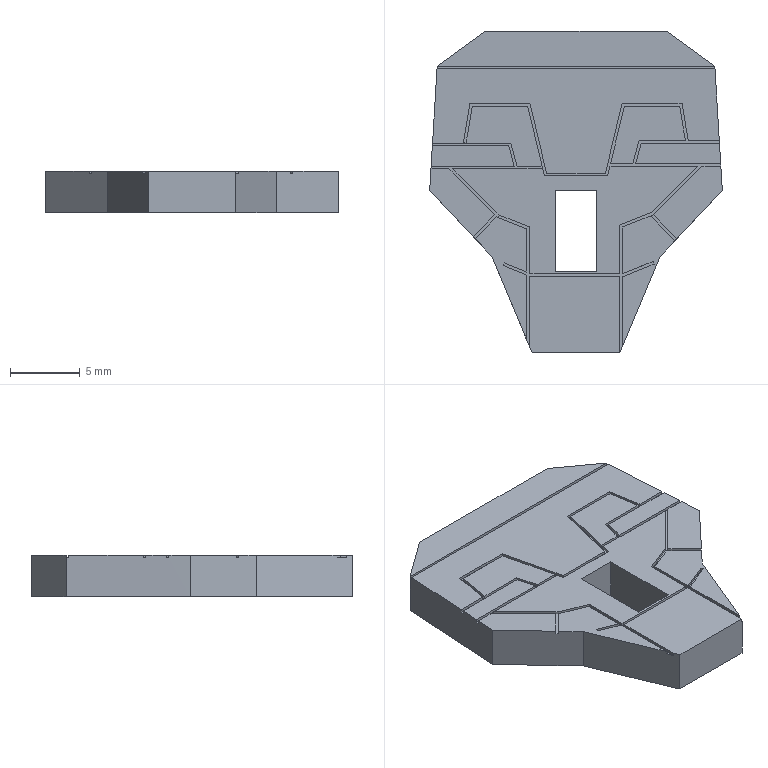Part | SolidWorks | features BaseBody 1 | 1 solid | 105 faces | box 20.921 x 23.01 x 3 mm | volume 1032 mm3 | plane 97 | spline 8